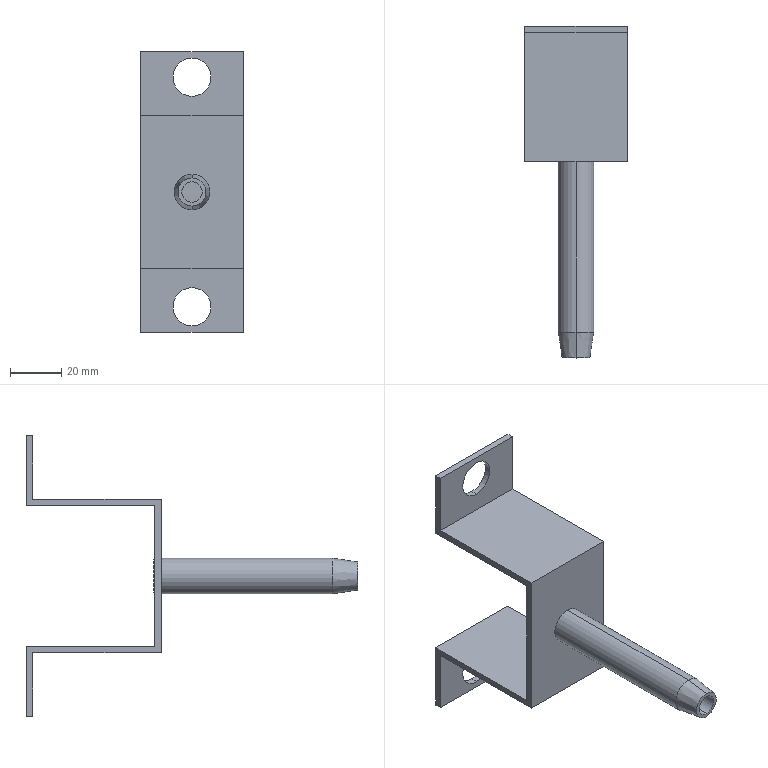Part | SolidWorks | features BaseBody 1 | 1 solid | 29 faces | box 40 x 130 x 110 mm | volume 31126 mm3 | plane 17 | cylinder 10 | cone 2 | commonest cylinder face diameters 15 x4 8 x2 13 x2 14 x2
STEP:
#1=CARTESIAN_POINT('',(861.946,-4005.973,2261.971));
#2=VERTEX_POINT('',#1);
#3=CARTESIAN_POINT('',(861.946,-4005.973,2247.971));
#4=VERTEX_POINT('',#3);
#5=CARTESIAN_POINT('',(861.946,-4005.973,2254.971));
#6=DIRECTION('',(0.,1.,0.));
#7=DIRECTION('',(0.,0.,-1.));
#8=AXIS2_PLACEMENT_3D('',#5,#6,#7);
#9=CIRCLE('',#8,7.);
#10=EDGE_CURVE('',#2,#4,#9,.T.);
#11=ORIENTED_EDGE('',*,*,#10,.F.);
#12=CARTESIAN_POINT('',(861.946,-4072.973,2261.971));
#13=VERTEX_POINT('',#12);
#14=CARTESIAN_POINT('',(861.946,-4039.473,2261.971));
#15=DIRECTION('',(0.,-1.,0.));
#16=VECTOR('',#15,1000.);
#17=LINE('',#14,#16);
#18=EDGE_CURVE('',#2,#13,#17,.T.);
#19=ORIENTED_EDGE('',*,*,#18,.T.);
#20=CARTESIAN_POINT('',(861.946,-4072.973,2247.971));
#21=VERTEX_POINT('',#20);
#22=CARTESIAN_POINT('',(861.946,-4072.973,2254.971));
#23=DIRECTION('',(0.,1.,0.));
#24=DIRECTION('',(0.,0.,-1.));
#25=AXIS2_PLACEMENT_3D('',#22,#23,#24);
#26=CIRCLE('',#25,7.);
#27=EDGE_CURVE('',#13,#21,#26,.T.);
#28=ORIENTED_EDGE('',*,*,#27,.T.);
#29=CARTESIAN_POINT('',(861.946,-4039.473,2247.971));
#30=DIRECTION('',(0.,-1.,0.));
#31=VECTOR('',#30,1000.);
#32=LINE('',#29,#31);
#33=EDGE_CURVE('',#4,#21,#32,.T.);
#34=ORIENTED_EDGE('',*,*,#33,.F.);
#35=EDGE_LOOP('',(#11,#19,#28,#34));
#36=FACE_OUTER_BOUND('',#35,.T.);
#37=CARTESIAN_POINT('',(861.946,-4039.473,2254.971));
#38=DIRECTION('',(0.,-1.,0.));
#39=DIRECTION('',(0.,0.,-1.));
#40=AXIS2_PLACEMENT_3D('',#37,#38,#39);
#41=CYLINDRICAL_SURFACE('',#40,7.);
#42=ADVANCED_FACE('',(#36),#41,.T.);
#43=CARTESIAN_POINT('',(861.946,-4082.973,2260.471));
#44=VERTEX_POINT('',#43);
#45=CARTESIAN_POINT('',(861.946,-4082.973,2249.471));
#46=VERTEX_POINT('',#45);
#47=CARTESIAN_POINT('',(861.946,-4082.973,2254.971));
#48=DIRECTION('',(0.,1.,0.));
#49=DIRECTION('',(0.,0.,1.));
#50=AXIS2_PLACEMENT_3D('',#47,#48,#49);
#51=CIRCLE('',#50,5.5);
#52=EDGE_CURVE('',#44,#46,#51,.T.);
#53=ORIENTED_EDGE('',*,*,#52,.T.);
#54=CARTESIAN_POINT('',(861.946,-4072.973,2247.971));
#55=DIRECTION('',(0.,0.9889,-0.1483));
#56=VECTOR('',#55,1000.);
#57=LINE('',#54,#56);
#58=EDGE_CURVE('',#46,#21,#57,.T.);
#59=ORIENTED_EDGE('',*,*,#58,.T.);
#60=ORIENTED_EDGE('',*,*,#27,.F.);
#61=CARTESIAN_POINT('',(861.946,-4072.973,2261.971));
#62=DIRECTION('',(0.,0.9889,0.1483));
#63=VECTOR('',#62,1000.);
#64=LINE('',#61,#63);
#65=EDGE_CURVE('',#44,#13,#64,.T.);
#66=ORIENTED_EDGE('',*,*,#65,.F.);
#67=EDGE_LOOP('',(#53,#59,#60,#66));
#68=FACE_OUTER_BOUND('',#67,.T.);
#69=CARTESIAN_POINT('',(861.946,-4072.973,2254.971));
#70=DIRECTION('',(0.,1.,0.));
#71=DIRECTION('',(0.,0.,1.));
#72=AXIS2_PLACEMENT_3D('',#69,#70,#71);
#73=CONICAL_SURFACE('',#72,7.,0.1489);
#74=ADVANCED_FACE('',(#68),#73,.T.);
#75=CARTESIAN_POINT('',(861.946,-3952.973,2307.471));
#76=VERTEX_POINT('',#75);
#77=CARTESIAN_POINT('',(861.946,-3952.973,2292.471));
#78=VERTEX_POINT('',#77);
#79=CARTESIAN_POINT('',(861.946,-3952.973,2299.971));
#80=DIRECTION('',(0.,-1.,0.));
#81=DIRECTION('',(0.,0.,-1.));
#82=AXIS2_PLACEMENT_3D('',#79,#80,#81);
#83=CIRCLE('',#82,7.5);
#84=EDGE_CURVE('',#76,#78,#83,.T.);
#85=ORIENTED_EDGE('',*,*,#84,.F.);
#86=CARTESIAN_POINT('',(861.946,-3955.473,2307.471));
#87=VERTEX_POINT('',#86);
#88=CARTESIAN_POINT('',(861.946,-3983.094,2307.471));
#89=DIRECTION('',(0.,-1.,0.));
#90=VECTOR('',#89,1000.);
#91=LINE('',#88,#90);
#92=EDGE_CURVE('',#76,#87,#91,.T.);
#93=ORIENTED_EDGE('',*,*,#92,.T.);
#94=CARTESIAN_POINT('',(861.946,-3955.473,2292.471));
#95=VERTEX_POINT('',#94);
#96=CARTESIAN_POINT('',(861.946,-3955.473,2299.971));
#97=DIRECTION('',(0.,1.,0.));
#98=DIRECTION('',(0.,0.,-1.));
#99=AXIS2_PLACEMENT_3D('',#96,#97,#98);
#100=CIRCLE('',#99,7.5);
#101=EDGE_CURVE('',#95,#87,#100,.T.);
#102=ORIENTED_EDGE('',*,*,#101,.F.);
#103=CARTESIAN_POINT('',(861.946,-3983.094,2292.471));
#104=DIRECTION('',(0.,-1.,0.));
#105=VECTOR('',#104,1000.);
#106=LINE('',#103,#105);
#107=EDGE_CURVE('',#78,#95,#106,.T.);
#108=ORIENTED_EDGE('',*,*,#107,.F.);
#109=EDGE_LOOP('',(#85,#93,#102,#108));
#110=FACE_OUTER_BOUND('',#109,.T.);
#111=CARTESIAN_POINT('',(861.946,-3983.094,2299.971));
#112=DIRECTION('',(0.,-1.,0.));
#113=DIRECTION('',(0.,0.,-1.));
#114=AXIS2_PLACEMENT_3D('',#111,#112,#113);
#115=CYLINDRICAL_SURFACE('',#114,7.5);
#116=ADVANCED_FACE('',(#110),#115,.F.);
#117=CARTESIAN_POINT('',(861.946,-3955.473,2202.471));
#118=VERTEX_POINT('',#117);
#119=CARTESIAN_POINT('',(861.946,-3955.473,2217.471));
#120=VERTEX_POINT('',#119);
#121=CARTESIAN_POINT('',(861.946,-3955.473,2209.971));
#122=DIRECTION('',(0.,1.,0.));
#123=DIRECTION('',(0.,0.,1.));
#124=AXIS2_PLACEMENT_3D('',#121,#122,#123);
#125=CIRCLE('',#124,7.5);
#126=EDGE_CURVE('',#118,#120,#125,.T.);
#127=ORIENTED_EDGE('',*,*,#126,.F.);
#128=CARTESIAN_POINT('',(861.946,-3952.973,2202.471));
#129=VERTEX_POINT('',#128);
#130=CARTESIAN_POINT('',(861.946,-3983.094,2202.471));
#131=DIRECTION('',(0.,1.,0.));
#132=VECTOR('',#131,1000.);
#133=LINE('',#130,#132);
#134=EDGE_CURVE('',#118,#129,#133,.T.);
#135=ORIENTED_EDGE('',*,*,#134,.T.);
#136=CARTESIAN_POINT('',(861.946,-3952.973,2217.471));
#137=VERTEX_POINT('',#136);
#138=CARTESIAN_POINT('',(861.946,-3952.973,2209.971));
#139=DIRECTION('',(0.,-1.,0.));
#140=DIRECTION('',(0.,0.,1.));
#141=AXIS2_PLACEMENT_3D('',#138,#139,#140);
#142=CIRCLE('',#141,7.5);
#143=EDGE_CURVE('',#137,#129,#142,.T.);
#144=ORIENTED_EDGE('',*,*,#143,.F.);
#145=CARTESIAN_POINT('',(861.946,-3983.094,2217.471));
#146=DIRECTION('',(0.,1.,0.));
#147=VECTOR('',#146,1000.);
#148=LINE('',#145,#147);
#149=EDGE_CURVE('',#120,#137,#148,.T.);
#150=ORIENTED_EDGE('',*,*,#149,.F.);
#151=EDGE_LOOP('',(#127,#135,#144,#150));
#152=FACE_OUTER_BOUND('',#151,.T.);
#153=CARTESIAN_POINT('',(861.946,-3983.094,2209.971));
#154=DIRECTION('',(0.,1.,0.));
#155=DIRECTION('',(0.,0.,1.));
#156=AXIS2_PLACEMENT_3D('',#153,#154,#155);
#157=CYLINDRICAL_SURFACE('',#156,7.5);
#158=ADVANCED_FACE('',(#152),#157,.F.);
#159=CARTESIAN_POINT('',(861.946,-4002.973,2248.471));
#160=VERTEX_POINT('',#159);
#161=CARTESIAN_POINT('',(861.946,-4002.973,2261.471));
#162=VERTEX_POINT('',#161);
#163=CARTESIAN_POINT('',(861.946,-4002.973,2254.971));
#164=DIRECTION('',(0.,-1.,0.));
#165=DIRECTION('',(0.,0.,-1.));
#166=AXIS2_PLACEMENT_3D('',#163,#164,#165);
#167=CIRCLE('',#166,6.5);
#168=EDGE_CURVE('',#160,#162,#167,.T.);
#169=ORIENTED_EDGE('',*,*,#168,.T.);
#170=CARTESIAN_POINT('',(861.946,-4003.473,2261.471));
#171=VERTEX_POINT('',#170);
#172=CARTESIAN_POINT('',(861.946,-4004.473,2261.471));
#173=DIRECTION('',(0.,-1.,0.));
#174=VECTOR('',#173,1000.);
#175=LINE('',#172,#174);
#176=EDGE_CURVE('',#162,#171,#175,.T.);
#177=ORIENTED_EDGE('',*,*,#176,.T.);
#178=CARTESIAN_POINT('',(861.946,-4003.473,2248.471));
#179=VERTEX_POINT('',#178);
#180=CARTESIAN_POINT('',(861.946,-4003.473,2254.971));
#181=DIRECTION('',(0.,-1.,0.));
#182=DIRECTION('',(0.,0.,-1.));
#183=AXIS2_PLACEMENT_3D('',#180,#181,#182);
#184=CIRCLE('',#183,6.5);
#185=EDGE_CURVE('',#179,#171,#184,.T.);
#186=ORIENTED_EDGE('',*,*,#185,.F.);
#187=CARTESIAN_POINT('',(861.946,-4004.473,2248.471));
#188=DIRECTION('',(0.,-1.,0.));
#189=VECTOR('',#188,1000.);
#190=LINE('',#187,#189);
#191=EDGE_CURVE('',#160,#179,#190,.T.);
#192=ORIENTED_EDGE('',*,*,#191,.F.);
#193=EDGE_LOOP('',(#169,#177,#186,#192));
#194=FACE_OUTER_BOUND('',#193,.T.);
#195=CARTESIAN_POINT('',(861.946,-4004.473,2254.971));
#196=DIRECTION('',(0.,-1.,0.));
#197=DIRECTION('',(0.,0.,-1.));
#198=AXIS2_PLACEMENT_3D('',#195,#196,#197);
#199=CYLINDRICAL_SURFACE('',#198,6.5);
#200=ADVANCED_FACE('',(#194),#199,.T.);
#201=CARTESIAN_POINT('',(861.946,-4068.973,2258.971));
#202=VERTEX_POINT('',#201);
#203=CARTESIAN_POINT('',(861.946,-4068.973,2250.971));
#204=VERTEX_POINT('',#203);
#205=CARTESIAN_POINT('',(861.946,-4068.973,2254.971));
#206=DIRECTION('',(0.,-1.,0.));
#207=DIRECTION('',(0.,0.,-1.));
#208=AXIS2_PLACEMENT_3D('',#205,#206,#207);
#209=CIRCLE('',#208,4.);
#210=EDGE_CURVE('',#202,#204,#209,.T.);
#211=ORIENTED_EDGE('',*,*,#210,.F.);
#212=CARTESIAN_POINT('',(861.946,-4082.973,2258.971));
#213=VERTEX_POINT('',#212);
#214=CARTESIAN_POINT('',(861.946,-4073.973,2258.971));
#215=DIRECTION('',(0.,-1.,0.));
#216=VECTOR('',#215,1000.);
#217=LINE('',#214,#216);
#218=EDGE_CURVE('',#202,#213,#217,.T.);
#219=ORIENTED_EDGE('',*,*,#218,.T.);
#220=CARTESIAN_POINT('',(861.946,-4082.973,2250.971));
#221=VERTEX_POINT('',#220);
#222=CARTESIAN_POINT('',(861.946,-4082.973,2254.971));
#223=DIRECTION('',(0.,1.,0.));
#224=DIRECTION('',(0.,0.,-1.));
#225=AXIS2_PLACEMENT_3D('',#222,#223,#224);
#226=CIRCLE('',#225,4.);
#227=EDGE_CURVE('',#221,#213,#226,.T.);
#228=ORIENTED_EDGE('',*,*,#227,.F.);
#229=CARTESIAN_POINT('',(861.946,-4073.973,2250.971));
#230=DIRECTION('',(0.,-1.,0.));
#231=VECTOR('',#230,1000.);
#232=LINE('',#229,#231);
#233=EDGE_CURVE('',#204,#221,#232,.T.);
#234=ORIENTED_EDGE('',*,*,#233,.F.);
#235=EDGE_LOOP('',(#211,#219,#228,#234));
#236=FACE_OUTER_BOUND('',#235,.T.);
#237=CARTESIAN_POINT('',(861.946,-4073.973,2254.971));
#238=DIRECTION('',(0.,-1.,0.));
#239=DIRECTION('',(0.,0.,-1.));
#240=AXIS2_PLACEMENT_3D('',#237,#238,#239);
#241=CYLINDRICAL_SURFACE('',#240,4.);
#242=ADVANCED_FACE('',(#236),#241,.F.);
#243=CARTESIAN_POINT('',(861.946,-4005.973,2254.971));
#244=DIRECTION('',(0.,1.,0.));
#245=DIRECTION('',(0.,0.,-1.));
#246=AXIS2_PLACEMENT_3D('',#243,#244,#245);
#247=CIRCLE('',#246,7.);
#248=EDGE_CURVE('',#4,#2,#247,.T.);
#249=ORIENTED_EDGE('',*,*,#248,.T.);
#250=ORIENTED_EDGE('',*,*,#10,.T.);
#251=EDGE_LOOP('',(#249,#250));
#252=FACE_BOUND('',#251,.T.);
#253=CARTESIAN_POINT('',(881.946,-4005.973,2224.971));
#254=VERTEX_POINT('',#253);
#255=CARTESIAN_POINT('',(881.946,-4005.973,2284.971));
#256=VERTEX_POINT('',#255);
#257=CARTESIAN_POINT('',(881.946,-4005.973,2284.971));
#258=DIRECTION('',(0.,0.,1.));
#259=VECTOR('',#258,1000.);
#260=LINE('',#257,#259);
#261=EDGE_CURVE('',#254,#256,#260,.T.);
#262=ORIENTED_EDGE('',*,*,#261,.T.);
#263=CARTESIAN_POINT('',(841.946,-4005.973,2284.971));
#264=VERTEX_POINT('',#263);
#265=CARTESIAN_POINT('',(876.946,-4005.973,2284.971));
#266=DIRECTION('',(-1.,0.,0.));
#267=VECTOR('',#266,1000.);
#268=LINE('',#265,#267);
#269=EDGE_CURVE('',#256,#264,#268,.T.);
#270=ORIENTED_EDGE('',*,*,#269,.T.);
#271=CARTESIAN_POINT('',(841.946,-4005.973,2224.971));
#272=VERTEX_POINT('',#271);
#273=CARTESIAN_POINT('',(841.946,-4005.973,2284.971));
#274=DIRECTION('',(0.,0.,-1.));
#275=VECTOR('',#274,1000.);
#276=LINE('',#273,#275);
#277=EDGE_CURVE('',#264,#272,#276,.T.);
#278=ORIENTED_EDGE('',*,*,#277,.T.);
#279=CARTESIAN_POINT('',(876.946,-4005.973,2224.971));
#280=DIRECTION('',(1.,0.,0.));
#281=VECTOR('',#280,1000.);
#282=LINE('',#279,#281);
#283=EDGE_CURVE('',#272,#254,#282,.T.);
#284=ORIENTED_EDGE('',*,*,#283,.T.);
#285=EDGE_LOOP('',(#262,#270,#278,#284));
#286=FACE_OUTER_BOUND('',#285,.T.);
#287=CARTESIAN_POINT('',(876.946,-4005.973,2284.971));
#288=DIRECTION('',(0.,-1.,0.));
#289=DIRECTION('',(0.,0.,-1.));
#290=AXIS2_PLACEMENT_3D('',#287,#288,#289);
#291=PLANE('',#290);
#292=ADVANCED_FACE('',(#252,#286),#291,.T.);
#293=ORIENTED_EDGE('',*,*,#18,.F.);
#294=ORIENTED_EDGE('',*,*,#248,.F.);
#295=ORIENTED_EDGE('',*,*,#33,.T.);
#296=CARTESIAN_POINT('',(861.946,-4072.973,2254.971));
#297=DIRECTION('',(0.,1.,0.));
#298=DIRECTION('',(0.,0.,-1.));
#299=AXIS2_PLACEMENT_3D('',#296,#297,#298);
#300=CIRCLE('',#299,7.);
#301=EDGE_CURVE('',#21,#13,#300,.T.);
#302=ORIENTED_EDGE('',*,*,#301,.T.);
#303=EDGE_LOOP('',(#293,#294,#295,#302));
#304=FACE_OUTER_BOUND('',#303,.T.);
#305=CARTESIAN_POINT('',(861.946,-4039.473,2254.971));
#306=DIRECTION('',(0.,-1.,0.));
#307=DIRECTION('',(0.,0.,-1.));
#308=AXIS2_PLACEMENT_3D('',#305,#306,#307);
#309=CYLINDRICAL_SURFACE('',#308,7.);
#310=ADVANCED_FACE('',(#304),#309,.T.);
#311=CARTESIAN_POINT('',(881.946,-3955.473,2284.971));
#312=VERTEX_POINT('',#311);
#313=CARTESIAN_POINT('',(881.946,-3955.473,2284.971));
#314=DIRECTION('',(0.,1.,0.));
#315=VECTOR('',#314,1000.);
#316=LINE('',#313,#315);
#317=EDGE_CURVE('',#256,#312,#316,.T.);
#318=ORIENTED_EDGE('',*,*,#317,.T.);
#319=CARTESIAN_POINT('',(841.946,-3955.473,2284.971));
#320=VERTEX_POINT('',#319);
#321=CARTESIAN_POINT('',(881.946,-3955.473,2284.971));
#322=DIRECTION('',(-1.,0.,0.));
#323=VECTOR('',#322,1000.);
#324=LINE('',#321,#323);
#325=EDGE_CURVE('',#312,#320,#324,.T.);
#326=ORIENTED_EDGE('',*,*,#325,.T.);
#327=CARTESIAN_POINT('',(841.946,-3955.473,2284.971));
#328=DIRECTION('',(0.,-1.,0.));
#329=VECTOR('',#328,1000.);
#330=LINE('',#327,#329);
#331=EDGE_CURVE('',#320,#264,#330,.T.);
#332=ORIENTED_EDGE('',*,*,#331,.T.);
#333=ORIENTED_EDGE('',*,*,#269,.F.);
#334=EDGE_LOOP('',(#318,#326,#332,#333));
#335=FACE_OUTER_BOUND('',#334,.T.);
#336=CARTESIAN_POINT('',(881.946,-3955.473,2284.971));
#337=DIRECTION('',(0.,0.,1.));
#338=DIRECTION('',(0.,-1.,0.));
#339=AXIS2_PLACEMENT_3D('',#336,#337,#338);
#340=PLANE('',#339);
#341=ADVANCED_FACE('',(#335),#340,.T.);
#342=CARTESIAN_POINT('',(881.946,-3955.473,2224.971));
#343=VERTEX_POINT('',#342);
#344=CARTESIAN_POINT('',(881.946,-3979.769,2224.971));
#345=DIRECTION('',(0.,1.,0.));
#346=VECTOR('',#345,1000.);
#347=LINE('',#344,#346);
#348=EDGE_CURVE('',#254,#343,#347,.T.);
#349=ORIENTED_EDGE('',*,*,#348,.T.);
#350=CARTESIAN_POINT('',(881.946,-3955.473,2199.971));
#351=VERTEX_POINT('',#350);
#352=CARTESIAN_POINT('',(881.946,-3955.473,2254.971));
#353=DIRECTION('',(0.,0.,-1.));
#354=VECTOR('',#353,1000.);
#355=LINE('',#352,#354);
#356=EDGE_CURVE('',#343,#351,#355,.T.);
#357=ORIENTED_EDGE('',*,*,#356,.T.);
#358=CARTESIAN_POINT('',(881.946,-3952.973,2199.971));
#359=VERTEX_POINT('',#358);
#360=CARTESIAN_POINT('',(881.946,-3979.769,2199.971));
#361=DIRECTION('',(0.,1.,0.));
#362=VECTOR('',#361,1000.);
#363=LINE('',#360,#362);
#364=EDGE_CURVE('',#351,#359,#363,.T.);
#365=ORIENTED_EDGE('',*,*,#364,.T.);
#366=CARTESIAN_POINT('',(881.946,-3952.973,2227.471));
#367=VERTEX_POINT('',#366);
#368=CARTESIAN_POINT('',(881.946,-3952.973,2254.971));
#369=DIRECTION('',(0.,0.,1.));
#370=VECTOR('',#369,1000.);
#371=LINE('',#368,#370);
#372=EDGE_CURVE('',#359,#367,#371,.T.);
#373=ORIENTED_EDGE('',*,*,#372,.T.);
#374=CARTESIAN_POINT('',(881.946,-4003.473,2227.471));
#375=VERTEX_POINT('',#374);
#376=CARTESIAN_POINT('',(881.946,-3979.769,2227.471));
#377=DIRECTION('',(0.,-1.,0.));
#378=VECTOR('',#377,1000.);
#379=LINE('',#376,#378);
#380=EDGE_CURVE('',#367,#375,#379,.T.);
#381=ORIENTED_EDGE('',*,*,#380,.T.);
#382=CARTESIAN_POINT('',(881.946,-4003.473,2282.471));
#383=VERTEX_POINT('',#382);
#384=CARTESIAN_POINT('',(881.946,-4003.473,2254.971));
#385=DIRECTION('',(0.,0.,1.));
#386=VECTOR('',#385,1000.);
#387=LINE('',#384,#386);
#388=EDGE_CURVE('',#375,#383,#387,.T.);
#389=ORIENTED_EDGE('',*,*,#388,.T.);
#390=CARTESIAN_POINT('',(881.946,-3952.973,2282.471));
#391=VERTEX_POINT('',#390);
#392=CARTESIAN_POINT('',(881.946,-3979.769,2282.471));
#393=DIRECTION('',(0.,1.,0.));
#394=VECTOR('',#393,1000.);
#395=LINE('',#392,#394);
#396=EDGE_CURVE('',#383,#391,#395,.T.);
#397=ORIENTED_EDGE('',*,*,#396,.T.);
#398=CARTESIAN_POINT('',(881.946,-3952.973,2309.971));
#399=VERTEX_POINT('',#398);
#400=CARTESIAN_POINT('',(881.946,-3952.973,2254.971));
#401=DIRECTION('',(0.,0.,1.));
#402=VECTOR('',#401,1000.);
#403=LINE('',#400,#402);
#404=EDGE_CURVE('',#391,#399,#403,.T.);
#405=ORIENTED_EDGE('',*,*,#404,.T.);
#406=CARTESIAN_POINT('',(881.946,-3955.473,2309.971));
#407=VERTEX_POINT('',#406);
#408=CARTESIAN_POINT('',(881.946,-3979.769,2309.971));
#409=DIRECTION('',(0.,-1.,0.));
#410=VECTOR('',#409,1000.);
#411=LINE('',#408,#410);
#412=EDGE_CURVE('',#399,#407,#411,.T.);
#413=ORIENTED_EDGE('',*,*,#412,.T.);
#414=CARTESIAN_POINT('',(881.946,-3955.473,2254.971));
#415=DIRECTION('',(0.,0.,-1.));
#416=VECTOR('',#415,1000.);
#417=LINE('',#414,#416);
#418=EDGE_CURVE('',#407,#312,#417,.T.);
#419=ORIENTED_EDGE('',*,*,#418,.T.);
#420=ORIENTED_EDGE('',*,*,#317,.F.);
#421=ORIENTED_EDGE('',*,*,#261,.F.);
#422=EDGE_LOOP('',(#349,#357,#365,#373,#381,#389,#397,#405,#413,#419,#420,#421));
#423=FACE_OUTER_BOUND('',#422,.T.);
#424=CARTESIAN_POINT('',(881.946,-3979.769,2254.971));
#425=DIRECTION('',(1.,0.,0.));
#426=DIRECTION('',(0.,0.,-1.));
#427=AXIS2_PLACEMENT_3D('',#424,#425,#426);
#428=PLANE('',#427);
#429=ADVANCED_FACE('',(#423),#428,.T.);
#430=ORIENTED_EDGE('',*,*,#348,.F.);
#431=ORIENTED_EDGE('',*,*,#283,.F.);
#432=CARTESIAN_POINT('',(841.946,-3955.473,2224.971));
#433=VERTEX_POINT('',#432);
#434=CARTESIAN_POINT('',(841.946,-4005.973,2224.971));
#435=DIRECTION('',(0.,1.,0.));
#436=VECTOR('',#435,1000.);
#437=LINE('',#434,#436);
#438=EDGE_CURVE('',#272,#433,#437,.T.);
#439=ORIENTED_EDGE('',*,*,#438,.T.);
#440=CARTESIAN_POINT('',(876.946,-3955.473,2224.971));
#441=DIRECTION('',(1.,0.,0.));
#442=VECTOR('',#441,1000.);
#443=LINE('',#440,#442);
#444=EDGE_CURVE('',#433,#343,#443,.T.);
#445=ORIENTED_EDGE('',*,*,#444,.T.);
#446=EDGE_LOOP('',(#430,#431,#439,#445));
#447=FACE_OUTER_BOUND('',#446,.T.);
#448=CARTESIAN_POINT('',(876.946,-4005.973,2224.971));
#449=DIRECTION('',(0.,0.,-1.));
#450=DIRECTION('',(-1.,0.,0.));
#451=AXIS2_PLACEMENT_3D('',#448,#449,#450);
#452=PLANE('',#451);
#453=ADVANCED_FACE('',(#447),#452,.T.);
#454=CARTESIAN_POINT('',(841.946,-3955.473,2199.971));
#455=VERTEX_POINT('',#454);
#456=CARTESIAN_POINT('',(841.946,-3952.973,2199.971));
#457=VERTEX_POINT('',#456);
#458=CARTESIAN_POINT('',(841.946,-3979.769,2199.971));
#459=DIRECTION('',(0.,1.,0.));
#460=VECTOR('',#459,1000.);
#461=LINE('',#458,#460);
#462=EDGE_CURVE('',#455,#457,#461,.T.);
#463=ORIENTED_EDGE('',*,*,#462,.F.);
#464=CARTESIAN_POINT('',(841.946,-3955.473,2254.971));
#465=DIRECTION('',(0.,0.,-1.));
#466=VECTOR('',#465,1000.);
#467=LINE('',#464,#466);
#468=EDGE_CURVE('',#433,#455,#467,.T.);
#469=ORIENTED_EDGE('',*,*,#468,.F.);
#470=ORIENTED_EDGE('',*,*,#438,.F.);
#471=ORIENTED_EDGE('',*,*,#277,.F.);
#472=ORIENTED_EDGE('',*,*,#331,.F.);
#473=CARTESIAN_POINT('',(841.946,-3955.473,2309.971));
#474=VERTEX_POINT('',#473);
#475=CARTESIAN_POINT('',(841.946,-3955.473,2254.971));
#476=DIRECTION('',(0.,0.,-1.));
#477=VECTOR('',#476,1000.);
#478=LINE('',#475,#477);
#479=EDGE_CURVE('',#474,#320,#478,.T.);
#480=ORIENTED_EDGE('',*,*,#479,.F.);
#481=CARTESIAN_POINT('',(841.946,-3952.973,2309.971));
#482=VERTEX_POINT('',#481);
#483=CARTESIAN_POINT('',(841.946,-3979.769,2309.971));
#484=DIRECTION('',(0.,-1.,0.));
#485=VECTOR('',#484,1000.);
#486=LINE('',#483,#485);
#487=EDGE_CURVE('',#482,#474,#486,.T.);
#488=ORIENTED_EDGE('',*,*,#487,.F.);
#489=CARTESIAN_POINT('',(841.946,-3952.973,2282.471));
#490=VERTEX_POINT('',#489);
#491=CARTESIAN_POINT('',(841.946,-3952.973,2254.971));
#492=DIRECTION('',(0.,0.,1.));
#493=VECTOR('',#492,1000.);
#494=LINE('',#491,#493);
#495=EDGE_CURVE('',#490,#482,#494,.T.);
#496=ORIENTED_EDGE('',*,*,#495,.F.);
#497=CARTESIAN_POINT('',(841.946,-4003.473,2282.471));
#498=VERTEX_POINT('',#497);
#499=CARTESIAN_POINT('',(841.946,-3979.769,2282.471));
#500=DIRECTION('',(0.,1.,0.));
#501=VECTOR('',#500,1000.);
#502=LINE('',#499,#501);
#503=EDGE_CURVE('',#498,#490,#502,.T.);
#504=ORIENTED_EDGE('',*,*,#503,.F.);
#505=CARTESIAN_POINT('',(841.946,-4003.473,2227.471));
#506=VERTEX_POINT('',#505);
#507=CARTESIAN_POINT('',(841.946,-4003.473,2254.971));
#508=DIRECTION('',(0.,0.,1.));
#509=VECTOR('',#508,1000.);
#510=LINE('',#507,#509);
#511=EDGE_CURVE('',#506,#498,#510,.T.);
#512=ORIENTED_EDGE('',*,*,#511,.F.);
#513=CARTESIAN_POINT('',(841.946,-3952.973,2227.471));
#514=VERTEX_POINT('',#513);
#515=CARTESIAN_POINT('',(841.946,-3979.769,2227.471));
#516=DIRECTION('',(0.,-1.,0.));
#517=VECTOR('',#516,1000.);
#518=LINE('',#515,#517);
#519=EDGE_CURVE('',#514,#506,#518,.T.);
#520=ORIENTED_EDGE('',*,*,#519,.F.);
#521=CARTESIAN_POINT('',(841.946,-3952.973,2254.971));
#522=DIRECTION('',(0.,0.,1.));
#523=VECTOR('',#522,1000.);
#524=LINE('',#521,#523);
#525=EDGE_CURVE('',#457,#514,#524,.T.);
#526=ORIENTED_EDGE('',*,*,#525,.F.);
#527=EDGE_LOOP('',(#463,#469,#470,#471,#472,#480,#488,#496,#504,#512,#520,#526));
#528=FACE_OUTER_BOUND('',#527,.T.);
#529=CARTESIAN_POINT('',(841.946,-3979.769,2254.971));
#530=DIRECTION('',(1.,0.,0.));
#531=DIRECTION('',(0.,0.,-1.));
#532=AXIS2_PLACEMENT_3D('',#529,#530,#531);
#533=PLANE('',#532);
#534=ADVANCED_FACE('',(#528),#533,.F.);
#535=ORIENTED_EDGE('',*,*,#58,.F.);
#536=CARTESIAN_POINT('',(861.946,-4082.973,2254.971));
#537=DIRECTION('',(0.,1.,0.));
#538=DIRECTION('',(0.,0.,1.));
#539=AXIS2_PLACEMENT_3D('',#536,#537,#538);
#540=CIRCLE('',#539,5.5);
#541=EDGE_CURVE('',#46,#44,#540,.T.);
#542=ORIENTED_EDGE('',*,*,#541,.T.);
#543=ORIENTED_EDGE('',*,*,#65,.T.);
#544=ORIENTED_EDGE('',*,*,#301,.F.);
#545=EDGE_LOOP('',(#535,#542,#543,#544));
#546=FACE_OUTER_BOUND('',#545,.T.);
#547=CARTESIAN_POINT('',(861.946,-4072.973,2254.971));
#548=DIRECTION('',(0.,1.,0.));
#549=DIRECTION('',(0.,0.,1.));
#550=AXIS2_PLACEMENT_3D('',#547,#548,#549);
#551=CONICAL_SURFACE('',#550,7.,0.1489);
#552=ADVANCED_FACE('',(#546),#551,.T.);
#553=ORIENTED_EDGE('',*,*,#418,.F.);
#554=CARTESIAN_POINT('',(876.946,-3955.473,2309.971));
#555=DIRECTION('',(-1.,0.,0.));
#556=VECTOR('',#555,1000.);
#557=LINE('',#554,#556);
#558=EDGE_CURVE('',#407,#474,#557,.T.);
#559=ORIENTED_EDGE('',*,*,#558,.T.);
#560=ORIENTED_EDGE('',*,*,#479,.T.);
#561=ORIENTED_EDGE('',*,*,#325,.F.);
#562=EDGE_LOOP('',(#553,#559,#560,#561));
#563=FACE_OUTER_BOUND('',#562,.T.);
#564=ORIENTED_EDGE('',*,*,#101,.T.);
#565=CARTESIAN_POINT('',(861.946,-3955.473,2299.971));
#566=DIRECTION('',(0.,1.,0.));
#567=DIRECTION('',(0.,0.,-1.));
#568=AXIS2_PLACEMENT_3D('',#565,#566,#567);
#569=CIRCLE('',#568,7.5);
#570=EDGE_CURVE('',#87,#95,#569,.T.);
#571=ORIENTED_EDGE('',*,*,#570,.T.);
#572=EDGE_LOOP('',(#564,#571));
#573=FACE_BOUND('',#572,.T.);
#574=CARTESIAN_POINT('',(876.946,-3955.473,2309.971));
#575=DIRECTION('',(0.,-1.,0.));
#576=DIRECTION('',(0.,0.,-1.));
#577=AXIS2_PLACEMENT_3D('',#574,#575,#576);
#578=PLANE('',#577);
#579=ADVANCED_FACE('',(#563,#573),#578,.T.);
#580=ORIENTED_EDGE('',*,*,#356,.F.);
#581=ORIENTED_EDGE('',*,*,#444,.F.);
#582=ORIENTED_EDGE('',*,*,#468,.T.);
#583=CARTESIAN_POINT('',(876.946,-3955.473,2199.971));
#584=DIRECTION('',(1.,0.,0.));
#585=VECTOR('',#584,1000.);
#586=LINE('',#583,#585);
#587=EDGE_CURVE('',#455,#351,#586,.T.);
#588=ORIENTED_EDGE('',*,*,#587,.T.);
#589=EDGE_LOOP('',(#580,#581,#582,#588));
#590=FACE_OUTER_BOUND('',#589,.T.);
#591=CARTESIAN_POINT('',(861.946,-3955.473,2209.971));
#592=DIRECTION('',(0.,1.,0.));
#593=DIRECTION('',(0.,0.,1.));
#594=AXIS2_PLACEMENT_3D('',#591,#592,#593);
#595=CIRCLE('',#594,7.5);
#596=EDGE_CURVE('',#120,#118,#595,.T.);
#597=ORIENTED_EDGE('',*,*,#596,.T.);
#598=ORIENTED_EDGE('',*,*,#126,.T.);
#599=EDGE_LOOP('',(#597,#598));
#600=FACE_BOUND('',#599,.T.);
#601=CARTESIAN_POINT('',(876.946,-3955.473,2224.971));
#602=DIRECTION('',(0.,-1.,0.));
#603=DIRECTION('',(0.,0.,-1.));
#604=AXIS2_PLACEMENT_3D('',#601,#602,#603);
#605=PLANE('',#604);
#606=ADVANCED_FACE('',(#590,#600),#605,.T.);
#607=ORIENTED_EDGE('',*,*,#412,.F.);
#608=CARTESIAN_POINT('',(876.946,-3952.973,2309.971));
#609=DIRECTION('',(-1.,0.,0.));
#610=VECTOR('',#609,1000.);
#611=LINE('',#608,#610);
#612=EDGE_CURVE('',#399,#482,#611,.T.);
#613=ORIENTED_EDGE('',*,*,#612,.T.);
#614=ORIENTED_EDGE('',*,*,#487,.T.);
#615=ORIENTED_EDGE('',*,*,#558,.F.);
#616=EDGE_LOOP('',(#607,#613,#614,#615));
#617=FACE_OUTER_BOUND('',#616,.T.);
#618=CARTESIAN_POINT('',(876.946,-3952.973,2309.971));
#619=DIRECTION('',(0.,0.,1.));
#620=DIRECTION('',(0.,-1.,0.));
#621=AXIS2_PLACEMENT_3D('',#618,#619,#620);
#622=PLANE('',#621);
#623=ADVANCED_FACE('',(#617),#622,.T.);
#624=ORIENTED_EDGE('',*,*,#404,.F.);
#625=CARTESIAN_POINT('',(876.946,-3952.973,2282.471));
#626=DIRECTION('',(-1.,0.,0.));
#627=VECTOR('',#626,1000.);
#628=LINE('',#625,#627);
#629=EDGE_CURVE('',#391,#490,#628,.T.);
#630=ORIENTED_EDGE('',*,*,#629,.T.);
#631=ORIENTED_EDGE('',*,*,#495,.T.);
#632=ORIENTED_EDGE('',*,*,#612,.F.);
#633=EDGE_LOOP('',(#624,#630,#631,#632));
#634=FACE_OUTER_BOUND('',#633,.T.);
#635=CARTESIAN_POINT('',(861.946,-3952.973,2299.971));
#636=DIRECTION('',(0.,-1.,0.));
#637=DIRECTION('',(0.,0.,-1.));
#638=AXIS2_PLACEMENT_3D('',#635,#636,#637);
#639=CIRCLE('',#638,7.5);
#640=EDGE_CURVE('',#78,#76,#639,.T.);
#641=ORIENTED_EDGE('',*,*,#640,.T.);
#642=ORIENTED_EDGE('',*,*,#84,.T.);
#643=EDGE_LOOP('',(#641,#642));
#644=FACE_BOUND('',#643,.T.);
#645=CARTESIAN_POINT('',(876.946,-3952.973,2282.471));
#646=DIRECTION('',(0.,1.,0.));
#647=DIRECTION('',(0.,0.,1.));
#648=AXIS2_PLACEMENT_3D('',#645,#646,#647);
#649=PLANE('',#648);
#650=ADVANCED_FACE('',(#634,#644),#649,.T.);
#651=ORIENTED_EDGE('',*,*,#396,.F.);
#652=CARTESIAN_POINT('',(876.946,-4003.473,2282.471));
#653=DIRECTION('',(-1.,0.,0.));
#654=VECTOR('',#653,1000.);
#655=LINE('',#652,#654);
#656=EDGE_CURVE('',#383,#498,#655,.T.);
#657=ORIENTED_EDGE('',*,*,#656,.T.);
#658=ORIENTED_EDGE('',*,*,#503,.T.);
#659=ORIENTED_EDGE('',*,*,#629,.F.);
#660=EDGE_LOOP('',(#651,#657,#658,#659));
#661=FACE_OUTER_BOUND('',#660,.T.);
#662=CARTESIAN_POINT('',(876.946,-4003.473,2282.471));
#663=DIRECTION('',(0.,0.,-1.));
#664=DIRECTION('',(-1.,0.,0.));
#665=AXIS2_PLACEMENT_3D('',#662,#663,#664);
#666=PLANE('',#665);
#667=ADVANCED_FACE('',(#661),#666,.T.);
#668=ORIENTED_EDGE('',*,*,#185,.T.);
#669=CARTESIAN_POINT('',(861.946,-4003.473,2254.971));
#670=DIRECTION('',(0.,-1.,0.));
#671=DIRECTION('',(0.,0.,-1.));
#672=AXIS2_PLACEMENT_3D('',#669,#670,#671);
#673=CIRCLE('',#672,6.5);
#674=EDGE_CURVE('',#171,#179,#673,.T.);
#675=ORIENTED_EDGE('',*,*,#674,.T.);
#676=EDGE_LOOP('',(#668,#675));
#677=FACE_BOUND('',#676,.T.);
#678=ORIENTED_EDGE('',*,*,#388,.F.);
#679=CARTESIAN_POINT('',(876.946,-4003.473,2227.471));
#680=DIRECTION('',(-1.,0.,0.));
#681=VECTOR('',#680,1000.);
#682=LINE('',#679,#681);
#683=EDGE_CURVE('',#375,#506,#682,.T.);
#684=ORIENTED_EDGE('',*,*,#683,.T.);
#685=ORIENTED_EDGE('',*,*,#511,.T.);
#686=ORIENTED_EDGE('',*,*,#656,.F.);
#687=EDGE_LOOP('',(#678,#684,#685,#686));
#688=FACE_OUTER_BOUND('',#687,.T.);
#689=CARTESIAN_POINT('',(876.946,-4003.473,2227.471));
#690=DIRECTION('',(0.,1.,0.));
#691=DIRECTION('',(0.,0.,1.));
#692=AXIS2_PLACEMENT_3D('',#689,#690,#691);
#693=PLANE('',#692);
#694=ADVANCED_FACE('',(#677,#688),#693,.T.);
#695=ORIENTED_EDGE('',*,*,#380,.F.);
#696=CARTESIAN_POINT('',(876.946,-3952.973,2227.471));
#697=DIRECTION('',(-1.,0.,0.));
#698=VECTOR('',#697,1000.);
#699=LINE('',#696,#698);
#700=EDGE_CURVE('',#367,#514,#699,.T.);
#701=ORIENTED_EDGE('',*,*,#700,.T.);
#702=ORIENTED_EDGE('',*,*,#519,.T.);
#703=ORIENTED_EDGE('',*,*,#683,.F.);
#704=EDGE_LOOP('',(#695,#701,#702,#703));
#705=FACE_OUTER_BOUND('',#704,.T.);
#706=CARTESIAN_POINT('',(876.946,-3952.973,2227.471));
#707=DIRECTION('',(0.,0.,1.));
#708=DIRECTION('',(0.,-1.,0.));
#709=AXIS2_PLACEMENT_3D('',#706,#707,#708);
#710=PLANE('',#709);
#711=ADVANCED_FACE('',(#705),#710,.T.);
#712=ORIENTED_EDGE('',*,*,#372,.F.);
#713=CARTESIAN_POINT('',(876.946,-3952.973,2199.971));
#714=DIRECTION('',(-1.,0.,0.));
#715=VECTOR('',#714,1000.);
#716=LINE('',#713,#715);
#717=EDGE_CURVE('',#359,#457,#716,.T.);
#718=ORIENTED_EDGE('',*,*,#717,.T.);
#719=ORIENTED_EDGE('',*,*,#525,.T.);
#720=ORIENTED_EDGE('',*,*,#700,.F.);
#721=EDGE_LOOP('',(#712,#718,#719,#720));
#722=FACE_OUTER_BOUND('',#721,.T.);
#723=ORIENTED_EDGE('',*,*,#143,.T.);
#724=CARTESIAN_POINT('',(861.946,-3952.973,2209.971));
#725=DIRECTION('',(0.,-1.,0.));
#726=DIRECTION('',(0.,0.,1.));
#727=AXIS2_PLACEMENT_3D('',#724,#725,#726);
#728=CIRCLE('',#727,7.5);
#729=EDGE_CURVE('',#129,#137,#728,.T.);
#730=ORIENTED_EDGE('',*,*,#729,.T.);
#731=EDGE_LOOP('',(#723,#730));
#732=FACE_BOUND('',#731,.T.);
#733=CARTESIAN_POINT('',(876.946,-3952.973,2199.971));
#734=DIRECTION('',(0.,1.,0.));
#735=DIRECTION('',(0.,0.,1.));
#736=AXIS2_PLACEMENT_3D('',#733,#734,#735);
#737=PLANE('',#736);
#738=ADVANCED_FACE('',(#722,#732),#737,.T.);
#739=ORIENTED_EDGE('',*,*,#364,.F.);
#740=ORIENTED_EDGE('',*,*,#587,.F.);
#741=ORIENTED_EDGE('',*,*,#462,.T.);
#742=ORIENTED_EDGE('',*,*,#717,.F.);
#743=EDGE_LOOP('',(#739,#740,#741,#742));
#744=FACE_OUTER_BOUND('',#743,.T.);
#745=CARTESIAN_POINT('',(876.946,-3955.473,2199.971));
#746=DIRECTION('',(0.,0.,-1.));
#747=DIRECTION('',(-1.,0.,0.));
#748=AXIS2_PLACEMENT_3D('',#745,#746,#747);
#749=PLANE('',#748);
#750=ADVANCED_FACE('',(#744),#749,.T.);
#751=ORIENTED_EDGE('',*,*,#52,.F.);
#752=ORIENTED_EDGE('',*,*,#541,.F.);
#753=EDGE_LOOP('',(#751,#752));
#754=FACE_OUTER_BOUND('',#753,.T.);
#755=ORIENTED_EDGE('',*,*,#227,.T.);
#756=CARTESIAN_POINT('',(861.946,-4082.973,2254.971));
#757=DIRECTION('',(0.,1.,0.));
#758=DIRECTION('',(0.,0.,-1.));
#759=AXIS2_PLACEMENT_3D('',#756,#757,#758);
#760=CIRCLE('',#759,4.);
#761=EDGE_CURVE('',#213,#221,#760,.T.);
#762=ORIENTED_EDGE('',*,*,#761,.T.);
#763=EDGE_LOOP('',(#755,#762));
#764=FACE_BOUND('',#763,.T.);
#765=CARTESIAN_POINT('',(861.946,-4082.973,2257.721));
#766=DIRECTION('',(0.,-1.,0.));
#767=DIRECTION('',(0.,0.,-1.));
#768=AXIS2_PLACEMENT_3D('',#765,#766,#767);
#769=PLANE('',#768);
#770=ADVANCED_FACE('',(#754,#764),#769,.T.);
#771=ORIENTED_EDGE('',*,*,#92,.F.);
#772=ORIENTED_EDGE('',*,*,#640,.F.);
#773=ORIENTED_EDGE('',*,*,#107,.T.);
#774=ORIENTED_EDGE('',*,*,#570,.F.);
#775=EDGE_LOOP('',(#771,#772,#773,#774));
#776=FACE_OUTER_BOUND('',#775,.T.);
#777=CARTESIAN_POINT('',(861.946,-3983.094,2299.971));
#778=DIRECTION('',(0.,-1.,0.));
#779=DIRECTION('',(0.,0.,-1.));
#780=AXIS2_PLACEMENT_3D('',#777,#778,#779);
#781=CYLINDRICAL_SURFACE('',#780,7.5);
#782=ADVANCED_FACE('',(#776),#781,.F.);
#783=ORIENTED_EDGE('',*,*,#134,.F.);
#784=ORIENTED_EDGE('',*,*,#596,.F.);
#785=ORIENTED_EDGE('',*,*,#149,.T.);
#786=ORIENTED_EDGE('',*,*,#729,.F.);
#787=EDGE_LOOP('',(#783,#784,#785,#786));
#788=FACE_OUTER_BOUND('',#787,.T.);
#789=CARTESIAN_POINT('',(861.946,-3983.094,2209.971));
#790=DIRECTION('',(0.,1.,0.));
#791=DIRECTION('',(0.,0.,1.));
#792=AXIS2_PLACEMENT_3D('',#789,#790,#791);
#793=CYLINDRICAL_SURFACE('',#792,7.5);
#794=ADVANCED_FACE('',(#788),#793,.F.);
#795=ORIENTED_EDGE('',*,*,#176,.F.);
#796=CARTESIAN_POINT('',(861.946,-4002.973,2254.971));
#797=DIRECTION('',(0.,-1.,0.));
#798=DIRECTION('',(0.,0.,-1.));
#799=AXIS2_PLACEMENT_3D('',#796,#797,#798);
#800=CIRCLE('',#799,6.5);
#801=EDGE_CURVE('',#162,#160,#800,.T.);
#802=ORIENTED_EDGE('',*,*,#801,.T.);
#803=ORIENTED_EDGE('',*,*,#191,.T.);
#804=ORIENTED_EDGE('',*,*,#674,.F.);
#805=EDGE_LOOP('',(#795,#802,#803,#804));
#806=FACE_OUTER_BOUND('',#805,.T.);
#807=CARTESIAN_POINT('',(861.946,-4004.473,2254.971));
#808=DIRECTION('',(0.,-1.,0.));
#809=DIRECTION('',(0.,0.,-1.));
#810=AXIS2_PLACEMENT_3D('',#807,#808,#809);
#811=CYLINDRICAL_SURFACE('',#810,6.5);
#812=ADVANCED_FACE('',(#806),#811,.T.);
#813=ORIENTED_EDGE('',*,*,#218,.F.);
#814=CARTESIAN_POINT('',(861.946,-4068.973,2254.971));
#815=DIRECTION('',(0.,-1.,0.));
#816=DIRECTION('',(0.,0.,-1.));
#817=AXIS2_PLACEMENT_3D('',#814,#815,#816);
#818=CIRCLE('',#817,4.);
#819=EDGE_CURVE('',#204,#202,#818,.T.);
#820=ORIENTED_EDGE('',*,*,#819,.F.);
#821=ORIENTED_EDGE('',*,*,#233,.T.);
#822=ORIENTED_EDGE('',*,*,#761,.F.);
#823=EDGE_LOOP('',(#813,#820,#821,#822));
#824=FACE_OUTER_BOUND('',#823,.T.);
#825=CARTESIAN_POINT('',(861.946,-4073.973,2254.971));
#826=DIRECTION('',(0.,-1.,0.));
#827=DIRECTION('',(0.,0.,-1.));
#828=AXIS2_PLACEMENT_3D('',#825,#826,#827);
#829=CYLINDRICAL_SURFACE('',#828,4.);
#830=ADVANCED_FACE('',(#824),#829,.F.);
#831=ORIENTED_EDGE('',*,*,#168,.F.);
#832=ORIENTED_EDGE('',*,*,#801,.F.);
#833=EDGE_LOOP('',(#831,#832));
#834=FACE_OUTER_BOUND('',#833,.T.);
#835=CARTESIAN_POINT('',(861.946,-4002.973,2258.221));
#836=DIRECTION('',(0.,1.,0.));
#837=DIRECTION('',(0.,0.,1.));
#838=AXIS2_PLACEMENT_3D('',#835,#836,#837);
#839=PLANE('',#838);
#840=ADVANCED_FACE('',(#834),#839,.T.);
#841=ORIENTED_EDGE('',*,*,#819,.T.);
#842=ORIENTED_EDGE('',*,*,#210,.T.);
#843=EDGE_LOOP('',(#841,#842));
#844=FACE_OUTER_BOUND('',#843,.T.);
#845=CARTESIAN_POINT('',(861.946,-4068.973,2254.971));
#846=DIRECTION('',(0.,1.,0.));
#847=DIRECTION('',(0.,0.,1.));
#848=AXIS2_PLACEMENT_3D('',#845,#846,#847);
#849=PLANE('',#848);
#850=ADVANCED_FACE('',(#844),#849,.F.);
#851=CLOSED_SHELL('',(#42,#74,#116,#158,#200,#242,#292,#310,#341,#429,#453,#534,#552,#579,#606,#623,#650,#667,#694,#711,#738,#750,#770,#782,#794,#812,#830,#840,#850));
#852=MANIFOLD_SOLID_BREP('',#851);
#853=CARTESIAN_POINT('',(0.,0.,0.));
#854=DIRECTION('',(0.,0.,1.));
#855=DIRECTION('',(1.,0.,0.));
#856=AXIS2_PLACEMENT_3D('',#853,#854,#855);
#857=(LENGTH_UNIT()NAMED_UNIT(*)SI_UNIT(.MILLI.,.METRE.));
#858=UNCERTAINTY_MEASURE_WITH_UNIT(LENGTH_MEASURE(0.00001),#857,'','');
#859=(NAMED_UNIT(*)PLANE_ANGLE_UNIT()SI_UNIT($,.RADIAN.));
#860=(NAMED_UNIT(*)SI_UNIT($,.STERADIAN.)SOLID_ANGLE_UNIT());
#861=(GEOMETRIC_REPRESENTATION_CONTEXT(3)GLOBAL_UNCERTAINTY_ASSIGNED_CONTEXT((#858))GLOBAL_UNIT_ASSIGNED_CONTEXT((#857,#859,#860))REPRESENTATION_CONTEXT('',''));
#862=ADVANCED_BREP_SHAPE_REPRESENTATION('',(#852,#856),#861);